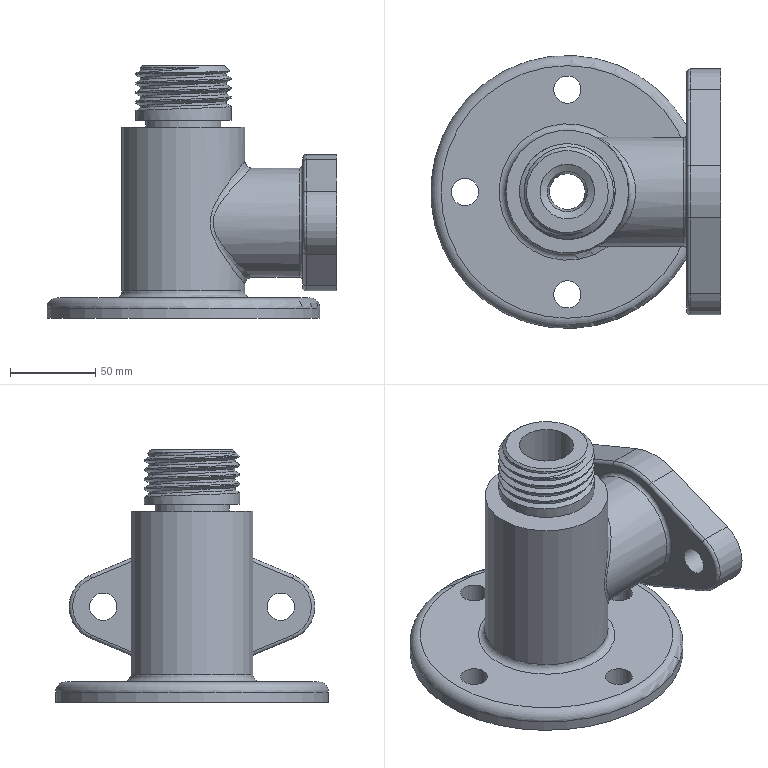Part | NX | features DATUM_CSYS 13, SKETCH 12, EXTRUDE 9, BLEND 4, CHAMFER 2, HOLE PACKAGE 2, SIMPLE HOLE 2, SWP104 1, SYMBOLIC_THREAD 1, THREADS 1 | 1 solid | 63 faces | box 170 x 160 x 148 mm | volume 670758 mm3 | cylinder 29 | plane 17 | torus 8 | cone 5 | spline 4 | commonest cylinder face diameters 16 x6 56 x5 4 x4 40 x2 44 x2 80 x2